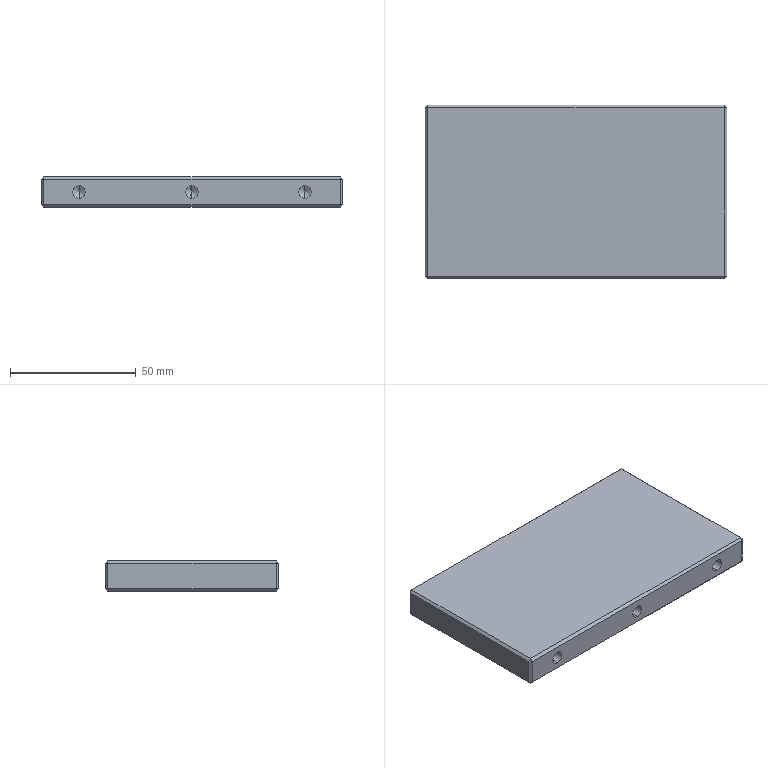Part | STEP file | 06-01-07 support plate | 1 solid | 49 faces | box 120 x 69 x 12 mm | volume 97250 mm3 | plane 27 | cylinder 12 | cone 10 | commonest cylinder face diameters 5 x6 4.2 x4 6 x2
STEP:
#1=CARTESIAN_POINT('',(0.,24.5,3.));
#2=VERTEX_POINT('',#1);
#3=CARTESIAN_POINT('',(0.,24.5,9.));
#4=VERTEX_POINT('',#3);
#5=CARTESIAN_POINT('',(0.,24.5,6.));
#6=DIRECTION('',(0.,1.,0.));
#7=DIRECTION('',(0.,0.,1.));
#8=AXIS2_PLACEMENT_3D('',#5,#6,#7);
#9=CIRCLE('',#8,3.);
#10=EDGE_CURVE('',#2,#4,#9,.T.);
#11=ORIENTED_EDGE('',*,*,#10,.F.);
#12=CARTESIAN_POINT('',(0.,34.5,3.));
#13=VERTEX_POINT('',#12);
#14=CARTESIAN_POINT('',(0.,24.5,3.));
#15=DIRECTION('',(0.,1.,0.));
#16=VECTOR('',#15,1000.);
#17=LINE('',#14,#16);
#18=EDGE_CURVE('',#2,#13,#17,.T.);
#19=ORIENTED_EDGE('',*,*,#18,.T.);
#20=CARTESIAN_POINT('',(0.,34.5,9.));
#21=VERTEX_POINT('',#20);
#22=CARTESIAN_POINT('',(0.,34.5,6.));
#23=DIRECTION('',(0.,1.,0.));
#24=DIRECTION('',(0.,0.,1.));
#25=AXIS2_PLACEMENT_3D('',#22,#23,#24);
#26=CIRCLE('',#25,3.);
#27=EDGE_CURVE('',#13,#21,#26,.T.);
#28=ORIENTED_EDGE('',*,*,#27,.T.);
#29=CARTESIAN_POINT('',(0.,24.5,9.));
#30=DIRECTION('',(0.,1.,0.));
#31=VECTOR('',#30,1000.);
#32=LINE('',#29,#31);
#33=EDGE_CURVE('',#4,#21,#32,.T.);
#34=ORIENTED_EDGE('',*,*,#33,.F.);
#35=EDGE_LOOP('',(#11,#19,#28,#34));
#36=FACE_OUTER_BOUND('',#35,.T.);
#37=CARTESIAN_POINT('',(0.,24.5,6.));
#38=DIRECTION('',(0.,1.,0.));
#39=DIRECTION('',(0.,0.,1.));
#40=AXIS2_PLACEMENT_3D('',#37,#38,#39);
#41=CYLINDRICAL_SURFACE('',#40,3.);
#42=ADVANCED_FACE('',(#36),#41,.F.);
#43=CARTESIAN_POINT('',(-14.5,20.5,3.9));
#44=VERTEX_POINT('',#43);
#45=CARTESIAN_POINT('',(-14.5,20.5,8.1));
#46=VERTEX_POINT('',#45);
#47=CARTESIAN_POINT('',(-14.5,20.5,6.));
#48=DIRECTION('',(0.,1.,0.));
#49=DIRECTION('',(0.,0.,1.));
#50=AXIS2_PLACEMENT_3D('',#47,#48,#49);
#51=CIRCLE('',#50,2.1);
#52=EDGE_CURVE('',#44,#46,#51,.T.);
#53=ORIENTED_EDGE('',*,*,#52,.F.);
#54=CARTESIAN_POINT('',(-14.5,34.5,3.9));
#55=VERTEX_POINT('',#54);
#56=CARTESIAN_POINT('',(-14.5,34.5,3.9));
#57=DIRECTION('',(0.,1.,0.));
#58=VECTOR('',#57,1000.);
#59=LINE('',#56,#58);
#60=EDGE_CURVE('',#44,#55,#59,.T.);
#61=ORIENTED_EDGE('',*,*,#60,.T.);
#62=CARTESIAN_POINT('',(-14.5,34.5,8.1));
#63=VERTEX_POINT('',#62);
#64=CARTESIAN_POINT('',(-14.5,34.5,6.));
#65=DIRECTION('',(0.,1.,0.));
#66=DIRECTION('',(0.,0.,1.));
#67=AXIS2_PLACEMENT_3D('',#64,#65,#66);
#68=CIRCLE('',#67,2.1);
#69=EDGE_CURVE('',#55,#63,#68,.T.);
#70=ORIENTED_EDGE('',*,*,#69,.T.);
#71=CARTESIAN_POINT('',(-14.5,34.5,8.1));
#72=DIRECTION('',(0.,1.,0.));
#73=VECTOR('',#72,1000.);
#74=LINE('',#71,#73);
#75=EDGE_CURVE('',#46,#63,#74,.T.);
#76=ORIENTED_EDGE('',*,*,#75,.F.);
#77=EDGE_LOOP('',(#53,#61,#70,#76));
#78=FACE_OUTER_BOUND('',#77,.T.);
#79=CARTESIAN_POINT('',(-14.5,34.5,6.));
#80=DIRECTION('',(0.,1.,0.));
#81=DIRECTION('',(0.,0.,1.));
#82=AXIS2_PLACEMENT_3D('',#79,#80,#81);
#83=CYLINDRICAL_SURFACE('',#82,2.1);
#84=ADVANCED_FACE('',(#78),#83,.F.);
#85=CARTESIAN_POINT('',(-14.5,19.238,6.));
#86=VERTEX_POINT('',#85);
#87=CARTESIAN_POINT('',(-14.5,20.5,8.1));
#88=DIRECTION('',(0.,0.515,0.8572));
#89=VECTOR('',#88,1000.);
#90=LINE('',#87,#89);
#91=EDGE_CURVE('',#86,#46,#90,.T.);
#92=ORIENTED_EDGE('',*,*,#91,.F.);
#93=CARTESIAN_POINT('',(-14.5,20.5,3.9));
#94=DIRECTION('',(0.,0.515,-0.8572));
#95=VECTOR('',#94,1000.);
#96=LINE('',#93,#95);
#97=EDGE_CURVE('',#86,#44,#96,.T.);
#98=ORIENTED_EDGE('',*,*,#97,.T.);
#99=ORIENTED_EDGE('',*,*,#52,.T.);
#100=EDGE_LOOP('',(#92,#98,#99));
#101=FACE_OUTER_BOUND('',#100,.T.);
#102=CARTESIAN_POINT('',(-14.5,20.5,6.));
#103=DIRECTION('',(0.,1.,0.));
#104=DIRECTION('',(0.,0.,1.));
#105=AXIS2_PLACEMENT_3D('',#102,#103,#104);
#106=CONICAL_SURFACE('',#105,2.1,1.03);
#107=ADVANCED_FACE('',(#101),#106,.F.);
#108=CARTESIAN_POINT('',(45.,20.5,3.9));
#109=VERTEX_POINT('',#108);
#110=CARTESIAN_POINT('',(45.,20.5,8.1));
#111=VERTEX_POINT('',#110);
#112=CARTESIAN_POINT('',(45.,20.5,6.));
#113=DIRECTION('',(0.,1.,0.));
#114=DIRECTION('',(0.,0.,1.));
#115=AXIS2_PLACEMENT_3D('',#112,#113,#114);
#116=CIRCLE('',#115,2.1);
#117=EDGE_CURVE('',#109,#111,#116,.T.);
#118=ORIENTED_EDGE('',*,*,#117,.F.);
#119=CARTESIAN_POINT('',(45.,34.5,3.9));
#120=VERTEX_POINT('',#119);
#121=CARTESIAN_POINT('',(45.,34.5,3.9));
#122=DIRECTION('',(0.,1.,0.));
#123=VECTOR('',#122,1000.);
#124=LINE('',#121,#123);
#125=EDGE_CURVE('',#109,#120,#124,.T.);
#126=ORIENTED_EDGE('',*,*,#125,.T.);
#127=CARTESIAN_POINT('',(45.,34.5,8.1));
#128=VERTEX_POINT('',#127);
#129=CARTESIAN_POINT('',(45.,34.5,6.));
#130=DIRECTION('',(0.,1.,0.));
#131=DIRECTION('',(0.,0.,1.));
#132=AXIS2_PLACEMENT_3D('',#129,#130,#131);
#133=CIRCLE('',#132,2.1);
#134=EDGE_CURVE('',#120,#128,#133,.T.);
#135=ORIENTED_EDGE('',*,*,#134,.T.);
#136=CARTESIAN_POINT('',(45.,34.5,8.1));
#137=DIRECTION('',(0.,1.,0.));
#138=VECTOR('',#137,1000.);
#139=LINE('',#136,#138);
#140=EDGE_CURVE('',#111,#128,#139,.T.);
#141=ORIENTED_EDGE('',*,*,#140,.F.);
#142=EDGE_LOOP('',(#118,#126,#135,#141));
#143=FACE_OUTER_BOUND('',#142,.T.);
#144=CARTESIAN_POINT('',(45.,34.5,6.));
#145=DIRECTION('',(0.,1.,0.));
#146=DIRECTION('',(0.,0.,1.));
#147=AXIS2_PLACEMENT_3D('',#144,#145,#146);
#148=CYLINDRICAL_SURFACE('',#147,2.1);
#149=ADVANCED_FACE('',(#143),#148,.F.);
#150=CARTESIAN_POINT('',(45.,19.238,6.));
#151=VERTEX_POINT('',#150);
#152=CARTESIAN_POINT('',(45.,20.5,8.1));
#153=DIRECTION('',(0.,0.515,0.8572));
#154=VECTOR('',#153,1000.);
#155=LINE('',#152,#154);
#156=EDGE_CURVE('',#151,#111,#155,.T.);
#157=ORIENTED_EDGE('',*,*,#156,.F.);
#158=CARTESIAN_POINT('',(45.,20.5,3.9));
#159=DIRECTION('',(0.,0.515,-0.8572));
#160=VECTOR('',#159,1000.);
#161=LINE('',#158,#160);
#162=EDGE_CURVE('',#151,#109,#161,.T.);
#163=ORIENTED_EDGE('',*,*,#162,.T.);
#164=ORIENTED_EDGE('',*,*,#117,.T.);
#165=EDGE_LOOP('',(#157,#163,#164));
#166=FACE_OUTER_BOUND('',#165,.T.);
#167=CARTESIAN_POINT('',(45.,20.5,6.));
#168=DIRECTION('',(0.,1.,0.));
#169=DIRECTION('',(0.,0.,1.));
#170=AXIS2_PLACEMENT_3D('',#167,#168,#169);
#171=CONICAL_SURFACE('',#170,2.1,1.03);
#172=ADVANCED_FACE('',(#166),#171,.F.);
#173=CARTESIAN_POINT('',(-45.,-17.5,8.5));
#174=VERTEX_POINT('',#173);
#175=CARTESIAN_POINT('',(-45.,-17.5,3.5));
#176=VERTEX_POINT('',#175);
#177=CARTESIAN_POINT('',(-45.,-17.5,6.));
#178=DIRECTION('',(0.,-1.,0.));
#179=DIRECTION('',(0.,0.,-1.));
#180=AXIS2_PLACEMENT_3D('',#177,#178,#179);
#181=CIRCLE('',#180,2.5);
#182=EDGE_CURVE('',#174,#176,#181,.T.);
#183=ORIENTED_EDGE('',*,*,#182,.F.);
#184=CARTESIAN_POINT('',(-45.,-34.5,8.5));
#185=VERTEX_POINT('',#184);
#186=CARTESIAN_POINT('',(-45.,-34.5,8.5));
#187=DIRECTION('',(0.,-1.,0.));
#188=VECTOR('',#187,1000.);
#189=LINE('',#186,#188);
#190=EDGE_CURVE('',#174,#185,#189,.T.);
#191=ORIENTED_EDGE('',*,*,#190,.T.);
#192=CARTESIAN_POINT('',(-45.,-34.5,3.5));
#193=VERTEX_POINT('',#192);
#194=CARTESIAN_POINT('',(-45.,-34.5,6.));
#195=DIRECTION('',(0.,-1.,0.));
#196=DIRECTION('',(0.,0.,-1.));
#197=AXIS2_PLACEMENT_3D('',#194,#195,#196);
#198=CIRCLE('',#197,2.5);
#199=EDGE_CURVE('',#185,#193,#198,.T.);
#200=ORIENTED_EDGE('',*,*,#199,.T.);
#201=CARTESIAN_POINT('',(-45.,-34.5,3.5));
#202=DIRECTION('',(0.,-1.,0.));
#203=VECTOR('',#202,1000.);
#204=LINE('',#201,#203);
#205=EDGE_CURVE('',#176,#193,#204,.T.);
#206=ORIENTED_EDGE('',*,*,#205,.F.);
#207=EDGE_LOOP('',(#183,#191,#200,#206));
#208=FACE_OUTER_BOUND('',#207,.T.);
#209=CARTESIAN_POINT('',(-45.,-34.5,6.));
#210=DIRECTION('',(0.,-1.,0.));
#211=DIRECTION('',(0.,0.,-1.));
#212=AXIS2_PLACEMENT_3D('',#209,#210,#211);
#213=CYLINDRICAL_SURFACE('',#212,2.5);
#214=ADVANCED_FACE('',(#208),#213,.F.);
#215=CARTESIAN_POINT('',(-45.,-15.998,6.));
#216=VERTEX_POINT('',#215);
#217=CARTESIAN_POINT('',(-45.,-17.5,3.5));
#218=DIRECTION('',(0.,-0.515,-0.8572));
#219=VECTOR('',#218,1000.);
#220=LINE('',#217,#219);
#221=EDGE_CURVE('',#216,#176,#220,.T.);
#222=ORIENTED_EDGE('',*,*,#221,.F.);
#223=CARTESIAN_POINT('',(-45.,-17.5,8.5));
#224=DIRECTION('',(0.,-0.515,0.8572));
#225=VECTOR('',#224,1000.);
#226=LINE('',#223,#225);
#227=EDGE_CURVE('',#216,#174,#226,.T.);
#228=ORIENTED_EDGE('',*,*,#227,.T.);
#229=ORIENTED_EDGE('',*,*,#182,.T.);
#230=EDGE_LOOP('',(#222,#228,#229));
#231=FACE_OUTER_BOUND('',#230,.T.);
#232=CARTESIAN_POINT('',(-45.,-17.5,6.));
#233=DIRECTION('',(0.,-1.,0.));
#234=DIRECTION('',(0.,0.,-1.));
#235=AXIS2_PLACEMENT_3D('',#232,#233,#234);
#236=CONICAL_SURFACE('',#235,2.5,1.03);
#237=ADVANCED_FACE('',(#231),#236,.F.);
#238=CARTESIAN_POINT('',(0.,-17.5,8.5));
#239=VERTEX_POINT('',#238);
#240=CARTESIAN_POINT('',(0.,-17.5,3.5));
#241=VERTEX_POINT('',#240);
#242=CARTESIAN_POINT('',(0.,-17.5,6.));
#243=DIRECTION('',(0.,-1.,0.));
#244=DIRECTION('',(0.,0.,-1.));
#245=AXIS2_PLACEMENT_3D('',#242,#243,#244);
#246=CIRCLE('',#245,2.5);
#247=EDGE_CURVE('',#239,#241,#246,.T.);
#248=ORIENTED_EDGE('',*,*,#247,.F.);
#249=CARTESIAN_POINT('',(0.,-34.5,8.5));
#250=VERTEX_POINT('',#249);
#251=CARTESIAN_POINT('',(0.,-34.5,8.5));
#252=DIRECTION('',(0.,-1.,0.));
#253=VECTOR('',#252,1000.);
#254=LINE('',#251,#253);
#255=EDGE_CURVE('',#239,#250,#254,.T.);
#256=ORIENTED_EDGE('',*,*,#255,.T.);
#257=CARTESIAN_POINT('',(0.,-34.5,3.5));
#258=VERTEX_POINT('',#257);
#259=CARTESIAN_POINT('',(0.,-34.5,6.));
#260=DIRECTION('',(0.,-1.,0.));
#261=DIRECTION('',(0.,0.,-1.));
#262=AXIS2_PLACEMENT_3D('',#259,#260,#261);
#263=CIRCLE('',#262,2.5);
#264=EDGE_CURVE('',#250,#258,#263,.T.);
#265=ORIENTED_EDGE('',*,*,#264,.T.);
#266=CARTESIAN_POINT('',(0.,-34.5,3.5));
#267=DIRECTION('',(0.,-1.,0.));
#268=VECTOR('',#267,1000.);
#269=LINE('',#266,#268);
#270=EDGE_CURVE('',#241,#258,#269,.T.);
#271=ORIENTED_EDGE('',*,*,#270,.F.);
#272=EDGE_LOOP('',(#248,#256,#265,#271));
#273=FACE_OUTER_BOUND('',#272,.T.);
#274=CARTESIAN_POINT('',(0.,-34.5,6.));
#275=DIRECTION('',(0.,-1.,0.));
#276=DIRECTION('',(0.,0.,-1.));
#277=AXIS2_PLACEMENT_3D('',#274,#275,#276);
#278=CYLINDRICAL_SURFACE('',#277,2.5);
#279=ADVANCED_FACE('',(#273),#278,.F.);
#280=CARTESIAN_POINT('',(0.,-15.998,6.));
#281=VERTEX_POINT('',#280);
#282=CARTESIAN_POINT('',(0.,-17.5,3.5));
#283=DIRECTION('',(0.,-0.515,-0.8572));
#284=VECTOR('',#283,1000.);
#285=LINE('',#282,#284);
#286=EDGE_CURVE('',#281,#241,#285,.T.);
#287=ORIENTED_EDGE('',*,*,#286,.F.);
#288=CARTESIAN_POINT('',(0.,-17.5,8.5));
#289=DIRECTION('',(0.,-0.515,0.8572));
#290=VECTOR('',#289,1000.);
#291=LINE('',#288,#290);
#292=EDGE_CURVE('',#281,#239,#291,.T.);
#293=ORIENTED_EDGE('',*,*,#292,.T.);
#294=ORIENTED_EDGE('',*,*,#247,.T.);
#295=EDGE_LOOP('',(#287,#293,#294));
#296=FACE_OUTER_BOUND('',#295,.T.);
#297=CARTESIAN_POINT('',(0.,-17.5,6.));
#298=DIRECTION('',(0.,-1.,0.));
#299=DIRECTION('',(0.,0.,-1.));
#300=AXIS2_PLACEMENT_3D('',#297,#298,#299);
#301=CONICAL_SURFACE('',#300,2.5,1.03);
#302=ADVANCED_FACE('',(#296),#301,.F.);
#303=CARTESIAN_POINT('',(45.,-17.5,8.5));
#304=VERTEX_POINT('',#303);
#305=CARTESIAN_POINT('',(45.,-17.5,3.5));
#306=VERTEX_POINT('',#305);
#307=CARTESIAN_POINT('',(45.,-17.5,6.));
#308=DIRECTION('',(0.,-1.,0.));
#309=DIRECTION('',(0.,0.,-1.));
#310=AXIS2_PLACEMENT_3D('',#307,#308,#309);
#311=CIRCLE('',#310,2.5);
#312=EDGE_CURVE('',#304,#306,#311,.T.);
#313=ORIENTED_EDGE('',*,*,#312,.F.);
#314=CARTESIAN_POINT('',(45.,-34.5,8.5));
#315=VERTEX_POINT('',#314);
#316=CARTESIAN_POINT('',(45.,-34.5,8.5));
#317=DIRECTION('',(0.,-1.,0.));
#318=VECTOR('',#317,1000.);
#319=LINE('',#316,#318);
#320=EDGE_CURVE('',#304,#315,#319,.T.);
#321=ORIENTED_EDGE('',*,*,#320,.T.);
#322=CARTESIAN_POINT('',(45.,-34.5,3.5));
#323=VERTEX_POINT('',#322);
#324=CARTESIAN_POINT('',(45.,-34.5,6.));
#325=DIRECTION('',(0.,-1.,0.));
#326=DIRECTION('',(0.,0.,-1.));
#327=AXIS2_PLACEMENT_3D('',#324,#325,#326);
#328=CIRCLE('',#327,2.5);
#329=EDGE_CURVE('',#315,#323,#328,.T.);
#330=ORIENTED_EDGE('',*,*,#329,.T.);
#331=CARTESIAN_POINT('',(45.,-34.5,3.5));
#332=DIRECTION('',(0.,-1.,0.));
#333=VECTOR('',#332,1000.);
#334=LINE('',#331,#333);
#335=EDGE_CURVE('',#306,#323,#334,.T.);
#336=ORIENTED_EDGE('',*,*,#335,.F.);
#337=EDGE_LOOP('',(#313,#321,#330,#336));
#338=FACE_OUTER_BOUND('',#337,.T.);
#339=CARTESIAN_POINT('',(45.,-34.5,6.));
#340=DIRECTION('',(0.,-1.,0.));
#341=DIRECTION('',(0.,0.,-1.));
#342=AXIS2_PLACEMENT_3D('',#339,#340,#341);
#343=CYLINDRICAL_SURFACE('',#342,2.5);
#344=ADVANCED_FACE('',(#338),#343,.F.);
#345=CARTESIAN_POINT('',(45.,-15.998,6.));
#346=VERTEX_POINT('',#345);
#347=CARTESIAN_POINT('',(45.,-17.5,3.5));
#348=DIRECTION('',(0.,-0.515,-0.8572));
#349=VECTOR('',#348,1000.);
#350=LINE('',#347,#349);
#351=EDGE_CURVE('',#346,#306,#350,.T.);
#352=ORIENTED_EDGE('',*,*,#351,.F.);
#353=CARTESIAN_POINT('',(45.,-17.5,8.5));
#354=DIRECTION('',(0.,-0.515,0.8572));
#355=VECTOR('',#354,1000.);
#356=LINE('',#353,#355);
#357=EDGE_CURVE('',#346,#304,#356,.T.);
#358=ORIENTED_EDGE('',*,*,#357,.T.);
#359=ORIENTED_EDGE('',*,*,#312,.T.);
#360=EDGE_LOOP('',(#352,#358,#359));
#361=FACE_OUTER_BOUND('',#360,.T.);
#362=CARTESIAN_POINT('',(45.,-17.5,6.));
#363=DIRECTION('',(0.,-1.,0.));
#364=DIRECTION('',(0.,0.,-1.));
#365=AXIS2_PLACEMENT_3D('',#362,#363,#364);
#366=CONICAL_SURFACE('',#365,2.5,1.03);
#367=ADVANCED_FACE('',(#361),#366,.F.);
#368=CARTESIAN_POINT('',(60.,-33.5,11.));
#369=VERTEX_POINT('',#368);
#370=CARTESIAN_POINT('',(60.,-33.5,1.));
#371=VERTEX_POINT('',#370);
#372=CARTESIAN_POINT('',(60.,-33.5,12.));
#373=DIRECTION('',(0.,0.,-1.));
#374=VECTOR('',#373,1000.);
#375=LINE('',#372,#374);
#376=EDGE_CURVE('',#369,#371,#375,.T.);
#377=ORIENTED_EDGE('',*,*,#376,.T.);
#378=CARTESIAN_POINT('',(60.,33.5,1.));
#379=VERTEX_POINT('',#378);
#380=CARTESIAN_POINT('',(60.,34.5,1.));
#381=DIRECTION('',(0.,1.,0.));
#382=VECTOR('',#381,1000.);
#383=LINE('',#380,#382);
#384=EDGE_CURVE('',#371,#379,#383,.T.);
#385=ORIENTED_EDGE('',*,*,#384,.T.);
#386=CARTESIAN_POINT('',(60.,33.5,11.));
#387=VERTEX_POINT('',#386);
#388=CARTESIAN_POINT('',(60.,33.5,12.));
#389=DIRECTION('',(0.,0.,1.));
#390=VECTOR('',#389,1000.);
#391=LINE('',#388,#390);
#392=EDGE_CURVE('',#379,#387,#391,.T.);
#393=ORIENTED_EDGE('',*,*,#392,.T.);
#394=CARTESIAN_POINT('',(60.,-34.5,11.));
#395=DIRECTION('',(0.,-1.,0.));
#396=VECTOR('',#395,1000.);
#397=LINE('',#394,#396);
#398=EDGE_CURVE('',#387,#369,#397,.T.);
#399=ORIENTED_EDGE('',*,*,#398,.T.);
#400=EDGE_LOOP('',(#377,#385,#393,#399));
#401=FACE_OUTER_BOUND('',#400,.T.);
#402=CARTESIAN_POINT('',(60.,34.5,12.));
#403=DIRECTION('',(-1.,0.,0.));
#404=DIRECTION('',(0.,-1.,0.));
#405=AXIS2_PLACEMENT_3D('',#402,#403,#404);
#406=PLANE('',#405);
#407=ADVANCED_FACE('',(#401),#406,.F.);
#408=CARTESIAN_POINT('',(59.,34.5,11.));
#409=VERTEX_POINT('',#408);
#410=CARTESIAN_POINT('',(59.,34.5,1.));
#411=VERTEX_POINT('',#410);
#412=CARTESIAN_POINT('',(59.,34.5,12.));
#413=DIRECTION('',(0.,0.,-1.));
#414=VECTOR('',#413,1000.);
#415=LINE('',#412,#414);
#416=EDGE_CURVE('',#409,#411,#415,.T.);
#417=ORIENTED_EDGE('',*,*,#416,.T.);
#418=CARTESIAN_POINT('',(-59.,34.5,1.));
#419=VERTEX_POINT('',#418);
#420=CARTESIAN_POINT('',(-60.,34.5,1.));
#421=DIRECTION('',(-1.,0.,0.));
#422=VECTOR('',#421,1000.);
#423=LINE('',#420,#422);
#424=EDGE_CURVE('',#411,#419,#423,.T.);
#425=ORIENTED_EDGE('',*,*,#424,.T.);
#426=CARTESIAN_POINT('',(-59.,34.5,11.));
#427=VERTEX_POINT('',#426);
#428=CARTESIAN_POINT('',(-59.,34.5,12.));
#429=DIRECTION('',(0.,0.,1.));
#430=VECTOR('',#429,1000.);
#431=LINE('',#428,#430);
#432=EDGE_CURVE('',#419,#427,#431,.T.);
#433=ORIENTED_EDGE('',*,*,#432,.T.);
#434=CARTESIAN_POINT('',(60.,34.5,11.));
#435=DIRECTION('',(1.,0.,0.));
#436=VECTOR('',#435,1000.);
#437=LINE('',#434,#436);
#438=EDGE_CURVE('',#427,#409,#437,.T.);
#439=ORIENTED_EDGE('',*,*,#438,.T.);
#440=EDGE_LOOP('',(#417,#425,#433,#439));
#441=FACE_OUTER_BOUND('',#440,.T.);
#442=CARTESIAN_POINT('',(0.,34.5,6.));
#443=DIRECTION('',(0.,1.,0.));
#444=DIRECTION('',(0.,0.,1.));
#445=AXIS2_PLACEMENT_3D('',#442,#443,#444);
#446=CIRCLE('',#445,3.);
#447=EDGE_CURVE('',#21,#13,#446,.T.);
#448=ORIENTED_EDGE('',*,*,#447,.F.);
#449=ORIENTED_EDGE('',*,*,#27,.F.);
#450=EDGE_LOOP('',(#448,#449));
#451=FACE_BOUND('',#450,.T.);
#452=CARTESIAN_POINT('',(-14.5,34.5,6.));
#453=DIRECTION('',(0.,1.,0.));
#454=DIRECTION('',(0.,0.,1.));
#455=AXIS2_PLACEMENT_3D('',#452,#453,#454);
#456=CIRCLE('',#455,2.1);
#457=EDGE_CURVE('',#63,#55,#456,.T.);
#458=ORIENTED_EDGE('',*,*,#457,.F.);
#459=ORIENTED_EDGE('',*,*,#69,.F.);
#460=EDGE_LOOP('',(#458,#459));
#461=FACE_BOUND('',#460,.T.);
#462=CARTESIAN_POINT('',(45.,34.5,6.));
#463=DIRECTION('',(0.,1.,0.));
#464=DIRECTION('',(0.,0.,1.));
#465=AXIS2_PLACEMENT_3D('',#462,#463,#464);
#466=CIRCLE('',#465,2.1);
#467=EDGE_CURVE('',#128,#120,#466,.T.);
#468=ORIENTED_EDGE('',*,*,#467,.F.);
#469=ORIENTED_EDGE('',*,*,#134,.F.);
#470=EDGE_LOOP('',(#468,#469));
#471=FACE_BOUND('',#470,.T.);
#472=CARTESIAN_POINT('',(-60.,34.5,12.));
#473=DIRECTION('',(0.,-1.,0.));
#474=DIRECTION('',(0.,0.,-1.));
#475=AXIS2_PLACEMENT_3D('',#472,#473,#474);
#476=PLANE('',#475);
#477=ADVANCED_FACE('',(#441,#451,#461,#471),#476,.F.);
#478=CARTESIAN_POINT('',(-60.,33.5,11.));
#479=VERTEX_POINT('',#478);
#480=CARTESIAN_POINT('',(-60.,33.5,1.));
#481=VERTEX_POINT('',#480);
#482=CARTESIAN_POINT('',(-60.,33.5,12.));
#483=DIRECTION('',(0.,0.,-1.));
#484=VECTOR('',#483,1000.);
#485=LINE('',#482,#484);
#486=EDGE_CURVE('',#479,#481,#485,.T.);
#487=ORIENTED_EDGE('',*,*,#486,.T.);
#488=CARTESIAN_POINT('',(-60.,-33.5,1.));
#489=VERTEX_POINT('',#488);
#490=CARTESIAN_POINT('',(-60.,34.5,1.));
#491=DIRECTION('',(0.,-1.,0.));
#492=VECTOR('',#491,1000.);
#493=LINE('',#490,#492);
#494=EDGE_CURVE('',#481,#489,#493,.T.);
#495=ORIENTED_EDGE('',*,*,#494,.T.);
#496=CARTESIAN_POINT('',(-60.,-33.5,11.));
#497=VERTEX_POINT('',#496);
#498=CARTESIAN_POINT('',(-60.,-33.5,12.));
#499=DIRECTION('',(0.,0.,1.));
#500=VECTOR('',#499,1000.);
#501=LINE('',#498,#500);
#502=EDGE_CURVE('',#489,#497,#501,.T.);
#503=ORIENTED_EDGE('',*,*,#502,.T.);
#504=CARTESIAN_POINT('',(-60.,34.5,11.));
#505=DIRECTION('',(0.,1.,0.));
#506=VECTOR('',#505,1000.);
#507=LINE('',#504,#506);
#508=EDGE_CURVE('',#497,#479,#507,.T.);
#509=ORIENTED_EDGE('',*,*,#508,.T.);
#510=EDGE_LOOP('',(#487,#495,#503,#509));
#511=FACE_OUTER_BOUND('',#510,.T.);
#512=CARTESIAN_POINT('',(-60.,34.5,12.));
#513=DIRECTION('',(1.,0.,0.));
#514=DIRECTION('',(0.,1.,0.));
#515=AXIS2_PLACEMENT_3D('',#512,#513,#514);
#516=PLANE('',#515);
#517=ADVANCED_FACE('',(#511),#516,.F.);
#518=CARTESIAN_POINT('',(59.,-34.5,11.));
#519=VERTEX_POINT('',#518);
#520=CARTESIAN_POINT('',(-59.,-34.5,11.));
#521=VERTEX_POINT('',#520);
#522=CARTESIAN_POINT('',(-60.,-34.5,11.));
#523=DIRECTION('',(-1.,0.,0.));
#524=VECTOR('',#523,1000.);
#525=LINE('',#522,#524);
#526=EDGE_CURVE('',#519,#521,#525,.T.);
#527=ORIENTED_EDGE('',*,*,#526,.T.);
#528=CARTESIAN_POINT('',(-59.,-34.5,1.));
#529=VERTEX_POINT('',#528);
#530=CARTESIAN_POINT('',(-59.,-34.5,12.));
#531=DIRECTION('',(0.,0.,-1.));
#532=VECTOR('',#531,1000.);
#533=LINE('',#530,#532);
#534=EDGE_CURVE('',#521,#529,#533,.T.);
#535=ORIENTED_EDGE('',*,*,#534,.T.);
#536=CARTESIAN_POINT('',(59.,-34.5,1.));
#537=VERTEX_POINT('',#536);
#538=CARTESIAN_POINT('',(-60.,-34.5,1.));
#539=DIRECTION('',(1.,0.,0.));
#540=VECTOR('',#539,1000.);
#541=LINE('',#538,#540);
#542=EDGE_CURVE('',#529,#537,#541,.T.);
#543=ORIENTED_EDGE('',*,*,#542,.T.);
#544=CARTESIAN_POINT('',(59.,-34.5,12.));
#545=DIRECTION('',(0.,0.,1.));
#546=VECTOR('',#545,1000.);
#547=LINE('',#544,#546);
#548=EDGE_CURVE('',#537,#519,#547,.T.);
#549=ORIENTED_EDGE('',*,*,#548,.T.);
#550=EDGE_LOOP('',(#527,#535,#543,#549));
#551=FACE_OUTER_BOUND('',#550,.T.);
#552=CARTESIAN_POINT('',(-45.,-34.5,6.));
#553=DIRECTION('',(0.,-1.,0.));
#554=DIRECTION('',(0.,0.,-1.));
#555=AXIS2_PLACEMENT_3D('',#552,#553,#554);
#556=CIRCLE('',#555,2.5);
#557=EDGE_CURVE('',#193,#185,#556,.T.);
#558=ORIENTED_EDGE('',*,*,#557,.F.);
#559=ORIENTED_EDGE('',*,*,#199,.F.);
#560=EDGE_LOOP('',(#558,#559));
#561=FACE_BOUND('',#560,.T.);
#562=CARTESIAN_POINT('',(0.,-34.5,6.));
#563=DIRECTION('',(0.,-1.,0.));
#564=DIRECTION('',(0.,0.,-1.));
#565=AXIS2_PLACEMENT_3D('',#562,#563,#564);
#566=CIRCLE('',#565,2.5);
#567=EDGE_CURVE('',#258,#250,#566,.T.);
#568=ORIENTED_EDGE('',*,*,#567,.F.);
#569=ORIENTED_EDGE('',*,*,#264,.F.);
#570=EDGE_LOOP('',(#568,#569));
#571=FACE_BOUND('',#570,.T.);
#572=CARTESIAN_POINT('',(45.,-34.5,6.));
#573=DIRECTION('',(0.,-1.,0.));
#574=DIRECTION('',(0.,0.,-1.));
#575=AXIS2_PLACEMENT_3D('',#572,#573,#574);
#576=CIRCLE('',#575,2.5);
#577=EDGE_CURVE('',#323,#315,#576,.T.);
#578=ORIENTED_EDGE('',*,*,#577,.F.);
#579=ORIENTED_EDGE('',*,*,#329,.F.);
#580=EDGE_LOOP('',(#578,#579));
#581=FACE_BOUND('',#580,.T.);
#582=CARTESIAN_POINT('',(-60.,-34.5,12.));
#583=DIRECTION('',(0.,1.,0.));
#584=DIRECTION('',(0.,0.,1.));
#585=AXIS2_PLACEMENT_3D('',#582,#583,#584);
#586=PLANE('',#585);
#587=ADVANCED_FACE('',(#551,#561,#571,#581),#586,.F.);
#588=CARTESIAN_POINT('',(-59.,33.5,12.));
#589=VERTEX_POINT('',#588);
#590=CARTESIAN_POINT('',(-59.,-33.5,12.));
#591=VERTEX_POINT('',#590);
#592=CARTESIAN_POINT('',(-59.,-34.5,12.));
#593=DIRECTION('',(0.,-1.,0.));
#594=VECTOR('',#593,1000.);
#595=LINE('',#592,#594);
#596=EDGE_CURVE('',#589,#591,#595,.T.);
#597=ORIENTED_EDGE('',*,*,#596,.T.);
#598=CARTESIAN_POINT('',(59.,-33.5,12.));
#599=VERTEX_POINT('',#598);
#600=CARTESIAN_POINT('',(60.,-33.5,12.));
#601=DIRECTION('',(1.,0.,0.));
#602=VECTOR('',#601,1000.);
#603=LINE('',#600,#602);
#604=EDGE_CURVE('',#591,#599,#603,.T.);
#605=ORIENTED_EDGE('',*,*,#604,.T.);
#606=CARTESIAN_POINT('',(59.,33.5,12.));
#607=VERTEX_POINT('',#606);
#608=CARTESIAN_POINT('',(59.,34.5,12.));
#609=DIRECTION('',(0.,1.,0.));
#610=VECTOR('',#609,1000.);
#611=LINE('',#608,#610);
#612=EDGE_CURVE('',#599,#607,#611,.T.);
#613=ORIENTED_EDGE('',*,*,#612,.T.);
#614=CARTESIAN_POINT('',(-60.,33.5,12.));
#615=DIRECTION('',(-1.,0.,0.));
#616=VECTOR('',#615,1000.);
#617=LINE('',#614,#616);
#618=EDGE_CURVE('',#607,#589,#617,.T.);
#619=ORIENTED_EDGE('',*,*,#618,.T.);
#620=EDGE_LOOP('',(#597,#605,#613,#619));
#621=FACE_OUTER_BOUND('',#620,.T.);
#622=CARTESIAN_POINT('',(60.,-34.5,12.));
#623=DIRECTION('',(0.,0.,1.));
#624=DIRECTION('',(1.,0.,0.));
#625=AXIS2_PLACEMENT_3D('',#622,#623,#624);
#626=PLANE('',#625);
#627=ADVANCED_FACE('',(#621),#626,.T.);
#628=CARTESIAN_POINT('',(-59.,-33.5,0.));
#629=VERTEX_POINT('',#628);
#630=CARTESIAN_POINT('',(-59.,33.5,0.));
#631=VERTEX_POINT('',#630);
#632=CARTESIAN_POINT('',(-59.,-34.5,0.));
#633=DIRECTION('',(0.,1.,0.));
#634=VECTOR('',#633,1000.);
#635=LINE('',#632,#634);
#636=EDGE_CURVE('',#629,#631,#635,.T.);
#637=ORIENTED_EDGE('',*,*,#636,.T.);
#638=CARTESIAN_POINT('',(59.,33.5,0.));
#639=VERTEX_POINT('',#638);
#640=CARTESIAN_POINT('',(60.,33.5,0.));
#641=DIRECTION('',(1.,0.,0.));
#642=VECTOR('',#641,1000.);
#643=LINE('',#640,#642);
#644=EDGE_CURVE('',#631,#639,#643,.T.);
#645=ORIENTED_EDGE('',*,*,#644,.T.);
#646=CARTESIAN_POINT('',(59.,-33.5,0.));
#647=VERTEX_POINT('',#646);
#648=CARTESIAN_POINT('',(59.,-34.5,0.));
#649=DIRECTION('',(0.,-1.,0.));
#650=VECTOR('',#649,1000.);
#651=LINE('',#648,#650);
#652=EDGE_CURVE('',#639,#647,#651,.T.);
#653=ORIENTED_EDGE('',*,*,#652,.T.);
#654=CARTESIAN_POINT('',(60.,-33.5,0.));
#655=DIRECTION('',(-1.,0.,0.));
#656=VECTOR('',#655,1000.);
#657=LINE('',#654,#656);
#658=EDGE_CURVE('',#647,#629,#657,.T.);
#659=ORIENTED_EDGE('',*,*,#658,.T.);
#660=EDGE_LOOP('',(#637,#645,#653,#659));
#661=FACE_OUTER_BOUND('',#660,.T.);
#662=CARTESIAN_POINT('',(60.,-34.5,0.));
#663=DIRECTION('',(0.,0.,1.));
#664=DIRECTION('',(1.,0.,0.));
#665=AXIS2_PLACEMENT_3D('',#662,#663,#664);
#666=PLANE('',#665);
#667=ADVANCED_FACE('',(#661),#666,.F.);
#668=ORIENTED_EDGE('',*,*,#357,.F.);
#669=ORIENTED_EDGE('',*,*,#351,.T.);
#670=CARTESIAN_POINT('',(45.,-17.5,6.));
#671=DIRECTION('',(0.,-1.,0.));
#672=DIRECTION('',(0.,0.,-1.));
#673=AXIS2_PLACEMENT_3D('',#670,#671,#672);
#674=CIRCLE('',#673,2.5);
#675=EDGE_CURVE('',#306,#304,#674,.T.);
#676=ORIENTED_EDGE('',*,*,#675,.T.);
#677=EDGE_LOOP('',(#668,#669,#676));
#678=FACE_OUTER_BOUND('',#677,.T.);
#679=CARTESIAN_POINT('',(45.,-17.5,6.));
#680=DIRECTION('',(0.,-1.,0.));
#681=DIRECTION('',(0.,0.,-1.));
#682=AXIS2_PLACEMENT_3D('',#679,#680,#681);
#683=CONICAL_SURFACE('',#682,2.5,1.03);
#684=ADVANCED_FACE('',(#678),#683,.F.);
#685=ORIENTED_EDGE('',*,*,#320,.F.);
#686=ORIENTED_EDGE('',*,*,#675,.F.);
#687=ORIENTED_EDGE('',*,*,#335,.T.);
#688=ORIENTED_EDGE('',*,*,#577,.T.);
#689=EDGE_LOOP('',(#685,#686,#687,#688));
#690=FACE_OUTER_BOUND('',#689,.T.);
#691=CARTESIAN_POINT('',(45.,-34.5,6.));
#692=DIRECTION('',(0.,-1.,0.));
#693=DIRECTION('',(0.,0.,-1.));
#694=AXIS2_PLACEMENT_3D('',#691,#692,#693);
#695=CYLINDRICAL_SURFACE('',#694,2.5);
#696=ADVANCED_FACE('',(#690),#695,.F.);
#697=ORIENTED_EDGE('',*,*,#292,.F.);
#698=ORIENTED_EDGE('',*,*,#286,.T.);
#699=CARTESIAN_POINT('',(0.,-17.5,6.));
#700=DIRECTION('',(0.,-1.,0.));
#701=DIRECTION('',(0.,0.,-1.));
#702=AXIS2_PLACEMENT_3D('',#699,#700,#701);
#703=CIRCLE('',#702,2.5);
#704=EDGE_CURVE('',#241,#239,#703,.T.);
#705=ORIENTED_EDGE('',*,*,#704,.T.);
#706=EDGE_LOOP('',(#697,#698,#705));
#707=FACE_OUTER_BOUND('',#706,.T.);
#708=CARTESIAN_POINT('',(0.,-17.5,6.));
#709=DIRECTION('',(0.,-1.,0.));
#710=DIRECTION('',(0.,0.,-1.));
#711=AXIS2_PLACEMENT_3D('',#708,#709,#710);
#712=CONICAL_SURFACE('',#711,2.5,1.03);
#713=ADVANCED_FACE('',(#707),#712,.F.);
#714=ORIENTED_EDGE('',*,*,#255,.F.);
#715=ORIENTED_EDGE('',*,*,#704,.F.);
#716=ORIENTED_EDGE('',*,*,#270,.T.);
#717=ORIENTED_EDGE('',*,*,#567,.T.);
#718=EDGE_LOOP('',(#714,#715,#716,#717));
#719=FACE_OUTER_BOUND('',#718,.T.);
#720=CARTESIAN_POINT('',(0.,-34.5,6.));
#721=DIRECTION('',(0.,-1.,0.));
#722=DIRECTION('',(0.,0.,-1.));
#723=AXIS2_PLACEMENT_3D('',#720,#721,#722);
#724=CYLINDRICAL_SURFACE('',#723,2.5);
#725=ADVANCED_FACE('',(#719),#724,.F.);
#726=ORIENTED_EDGE('',*,*,#227,.F.);
#727=ORIENTED_EDGE('',*,*,#221,.T.);
#728=CARTESIAN_POINT('',(-45.,-17.5,6.));
#729=DIRECTION('',(0.,-1.,0.));
#730=DIRECTION('',(0.,0.,-1.));
#731=AXIS2_PLACEMENT_3D('',#728,#729,#730);
#732=CIRCLE('',#731,2.5);
#733=EDGE_CURVE('',#176,#174,#732,.T.);
#734=ORIENTED_EDGE('',*,*,#733,.T.);
#735=EDGE_LOOP('',(#726,#727,#734));
#736=FACE_OUTER_BOUND('',#735,.T.);
#737=CARTESIAN_POINT('',(-45.,-17.5,6.));
#738=DIRECTION('',(0.,-1.,0.));
#739=DIRECTION('',(0.,0.,-1.));
#740=AXIS2_PLACEMENT_3D('',#737,#738,#739);
#741=CONICAL_SURFACE('',#740,2.5,1.03);
#742=ADVANCED_FACE('',(#736),#741,.F.);
#743=ORIENTED_EDGE('',*,*,#190,.F.);
#744=ORIENTED_EDGE('',*,*,#733,.F.);
#745=ORIENTED_EDGE('',*,*,#205,.T.);
#746=ORIENTED_EDGE('',*,*,#557,.T.);
#747=EDGE_LOOP('',(#743,#744,#745,#746));
#748=FACE_OUTER_BOUND('',#747,.T.);
#749=CARTESIAN_POINT('',(-45.,-34.5,6.));
#750=DIRECTION('',(0.,-1.,0.));
#751=DIRECTION('',(0.,0.,-1.));
#752=AXIS2_PLACEMENT_3D('',#749,#750,#751);
#753=CYLINDRICAL_SURFACE('',#752,2.5);
#754=ADVANCED_FACE('',(#748),#753,.F.);
#755=ORIENTED_EDGE('',*,*,#162,.F.);
#756=ORIENTED_EDGE('',*,*,#156,.T.);
#757=CARTESIAN_POINT('',(45.,20.5,6.));
#758=DIRECTION('',(0.,1.,0.));
#759=DIRECTION('',(0.,0.,1.));
#760=AXIS2_PLACEMENT_3D('',#757,#758,#759);
#761=CIRCLE('',#760,2.1);
#762=EDGE_CURVE('',#111,#109,#761,.T.);
#763=ORIENTED_EDGE('',*,*,#762,.T.);
#764=EDGE_LOOP('',(#755,#756,#763));
#765=FACE_OUTER_BOUND('',#764,.T.);
#766=CARTESIAN_POINT('',(45.,20.5,6.));
#767=DIRECTION('',(0.,1.,0.));
#768=DIRECTION('',(0.,0.,1.));
#769=AXIS2_PLACEMENT_3D('',#766,#767,#768);
#770=CONICAL_SURFACE('',#769,2.1,1.03);
#771=ADVANCED_FACE('',(#765),#770,.F.);
#772=ORIENTED_EDGE('',*,*,#125,.F.);
#773=ORIENTED_EDGE('',*,*,#762,.F.);
#774=ORIENTED_EDGE('',*,*,#140,.T.);
#775=ORIENTED_EDGE('',*,*,#467,.T.);
#776=EDGE_LOOP('',(#772,#773,#774,#775));
#777=FACE_OUTER_BOUND('',#776,.T.);
#778=CARTESIAN_POINT('',(45.,34.5,6.));
#779=DIRECTION('',(0.,1.,0.));
#780=DIRECTION('',(0.,0.,1.));
#781=AXIS2_PLACEMENT_3D('',#778,#779,#780);
#782=CYLINDRICAL_SURFACE('',#781,2.1);
#783=ADVANCED_FACE('',(#777),#782,.F.);
#784=ORIENTED_EDGE('',*,*,#97,.F.);
#785=ORIENTED_EDGE('',*,*,#91,.T.);
#786=CARTESIAN_POINT('',(-14.5,20.5,6.));
#787=DIRECTION('',(0.,1.,0.));
#788=DIRECTION('',(0.,0.,1.));
#789=AXIS2_PLACEMENT_3D('',#786,#787,#788);
#790=CIRCLE('',#789,2.1);
#791=EDGE_CURVE('',#46,#44,#790,.T.);
#792=ORIENTED_EDGE('',*,*,#791,.T.);
#793=EDGE_LOOP('',(#784,#785,#792));
#794=FACE_OUTER_BOUND('',#793,.T.);
#795=CARTESIAN_POINT('',(-14.5,20.5,6.));
#796=DIRECTION('',(0.,1.,0.));
#797=DIRECTION('',(0.,0.,1.));
#798=AXIS2_PLACEMENT_3D('',#795,#796,#797);
#799=CONICAL_SURFACE('',#798,2.1,1.03);
#800=ADVANCED_FACE('',(#794),#799,.F.);
#801=ORIENTED_EDGE('',*,*,#60,.F.);
#802=ORIENTED_EDGE('',*,*,#791,.F.);
#803=ORIENTED_EDGE('',*,*,#75,.T.);
#804=ORIENTED_EDGE('',*,*,#457,.T.);
#805=EDGE_LOOP('',(#801,#802,#803,#804));
#806=FACE_OUTER_BOUND('',#805,.T.);
#807=CARTESIAN_POINT('',(-14.5,34.5,6.));
#808=DIRECTION('',(0.,1.,0.));
#809=DIRECTION('',(0.,0.,1.));
#810=AXIS2_PLACEMENT_3D('',#807,#808,#809);
#811=CYLINDRICAL_SURFACE('',#810,2.1);
#812=ADVANCED_FACE('',(#806),#811,.F.);
#813=ORIENTED_EDGE('',*,*,#18,.F.);
#814=CARTESIAN_POINT('',(0.,24.5,6.));
#815=DIRECTION('',(0.,1.,0.));
#816=DIRECTION('',(0.,0.,1.));
#817=AXIS2_PLACEMENT_3D('',#814,#815,#816);
#818=CIRCLE('',#817,3.);
#819=EDGE_CURVE('',#4,#2,#818,.T.);
#820=ORIENTED_EDGE('',*,*,#819,.F.);
#821=ORIENTED_EDGE('',*,*,#33,.T.);
#822=ORIENTED_EDGE('',*,*,#447,.T.);
#823=EDGE_LOOP('',(#813,#820,#821,#822));
#824=FACE_OUTER_BOUND('',#823,.T.);
#825=CARTESIAN_POINT('',(0.,24.5,6.));
#826=DIRECTION('',(0.,1.,0.));
#827=DIRECTION('',(0.,0.,1.));
#828=AXIS2_PLACEMENT_3D('',#825,#826,#827);
#829=CYLINDRICAL_SURFACE('',#828,3.);
#830=ADVANCED_FACE('',(#824),#829,.F.);
#831=ORIENTED_EDGE('',*,*,#819,.T.);
#832=ORIENTED_EDGE('',*,*,#10,.T.);
#833=EDGE_LOOP('',(#831,#832));
#834=FACE_OUTER_BOUND('',#833,.T.);
#835=CARTESIAN_POINT('',(0.,24.5,6.));
#836=DIRECTION('',(0.,1.,0.));
#837=DIRECTION('',(0.,0.,1.));
#838=AXIS2_PLACEMENT_3D('',#835,#836,#837);
#839=PLANE('',#838);
#840=ADVANCED_FACE('',(#834),#839,.T.);
#841=CARTESIAN_POINT('',(59.,-33.5,12.));
#842=DIRECTION('',(0.,-0.7071,-0.7071));
#843=VECTOR('',#842,1000.);
#844=LINE('',#841,#843);
#845=EDGE_CURVE('',#599,#519,#844,.T.);
#846=ORIENTED_EDGE('',*,*,#845,.F.);
#847=ORIENTED_EDGE('',*,*,#604,.F.);
#848=CARTESIAN_POINT('',(-59.,-34.5,11.));
#849=DIRECTION('',(0.,0.7071,0.7071));
#850=VECTOR('',#849,1000.);
#851=LINE('',#848,#850);
#852=EDGE_CURVE('',#521,#591,#851,.T.);
#853=ORIENTED_EDGE('',*,*,#852,.F.);
#854=ORIENTED_EDGE('',*,*,#526,.F.);
#855=EDGE_LOOP('',(#846,#847,#853,#854));
#856=FACE_OUTER_BOUND('',#855,.T.);
#857=CARTESIAN_POINT('',(60.,-33.5,12.));
#858=DIRECTION('',(0.,-0.7071,0.7071));
#859=DIRECTION('',(0.,-0.7071,-0.7071));
#860=AXIS2_PLACEMENT_3D('',#857,#858,#859);
#861=PLANE('',#860);
#862=ADVANCED_FACE('',(#856),#861,.T.);
#863=CARTESIAN_POINT('',(59.,-33.5,12.));
#864=DIRECTION('',(0.7071,0.,-0.7071));
#865=VECTOR('',#864,1000.);
#866=LINE('',#863,#865);
#867=EDGE_CURVE('',#599,#369,#866,.T.);
#868=ORIENTED_EDGE('',*,*,#867,.F.);
#869=ORIENTED_EDGE('',*,*,#845,.T.);
#870=CARTESIAN_POINT('',(59.5,-34.,11.));
#871=DIRECTION('',(-0.7071,-0.7071,0.));
#872=VECTOR('',#871,1000.);
#873=LINE('',#870,#872);
#874=EDGE_CURVE('',#369,#519,#873,.T.);
#875=ORIENTED_EDGE('',*,*,#874,.F.);
#876=EDGE_LOOP('',(#868,#869,#875));
#877=FACE_OUTER_BOUND('',#876,.T.);
#878=CARTESIAN_POINT('',(59.,-33.5,12.));
#879=DIRECTION('',(0.5774,-0.5774,0.5774));
#880=DIRECTION('',(0.7071,0.7071,0.));
#881=AXIS2_PLACEMENT_3D('',#878,#879,#880);
#882=PLANE('',#881);
#883=ADVANCED_FACE('',(#877),#882,.T.);
#884=CARTESIAN_POINT('',(-59.,-34.5,11.));
#885=DIRECTION('',(-0.7071,0.7071,0.));
#886=VECTOR('',#885,1000.);
#887=LINE('',#884,#886);
#888=EDGE_CURVE('',#521,#497,#887,.T.);
#889=ORIENTED_EDGE('',*,*,#888,.F.);
#890=ORIENTED_EDGE('',*,*,#852,.T.);
#891=CARTESIAN_POINT('',(-59.5,-33.5,11.5));
#892=DIRECTION('',(0.7071,0.,0.7071));
#893=VECTOR('',#892,1000.);
#894=LINE('',#891,#893);
#895=EDGE_CURVE('',#497,#591,#894,.T.);
#896=ORIENTED_EDGE('',*,*,#895,.F.);
#897=EDGE_LOOP('',(#889,#890,#896));
#898=FACE_OUTER_BOUND('',#897,.T.);
#899=CARTESIAN_POINT('',(-59.,-34.5,11.));
#900=DIRECTION('',(-0.5774,-0.5774,0.5774));
#901=DIRECTION('',(0.,-0.7071,-0.7071));
#902=AXIS2_PLACEMENT_3D('',#899,#900,#901);
#903=PLANE('',#902);
#904=ADVANCED_FACE('',(#898),#903,.T.);
#905=ORIENTED_EDGE('',*,*,#874,.T.);
#906=ORIENTED_EDGE('',*,*,#548,.F.);
#907=CARTESIAN_POINT('',(59.,-34.5,1.));
#908=DIRECTION('',(-0.7071,-0.7071,0.));
#909=VECTOR('',#908,1000.);
#910=LINE('',#907,#909);
#911=EDGE_CURVE('',#371,#537,#910,.T.);
#912=ORIENTED_EDGE('',*,*,#911,.F.);
#913=ORIENTED_EDGE('',*,*,#376,.F.);
#914=EDGE_LOOP('',(#905,#906,#912,#913));
#915=FACE_OUTER_BOUND('',#914,.T.);
#916=CARTESIAN_POINT('',(60.,-33.5,12.));
#917=DIRECTION('',(-0.7071,0.7071,0.));
#918=DIRECTION('',(-0.7071,-0.7071,0.));
#919=AXIS2_PLACEMENT_3D('',#916,#917,#918);
#920=PLANE('',#919);
#921=ADVANCED_FACE('',(#915),#920,.F.);
#922=ORIENTED_EDGE('',*,*,#867,.T.);
#923=ORIENTED_EDGE('',*,*,#398,.F.);
#924=CARTESIAN_POINT('',(59.,33.5,12.));
#925=DIRECTION('',(0.7071,0.,-0.7071));
#926=VECTOR('',#925,1000.);
#927=LINE('',#924,#926);
#928=EDGE_CURVE('',#607,#387,#927,.T.);
#929=ORIENTED_EDGE('',*,*,#928,.F.);
#930=ORIENTED_EDGE('',*,*,#612,.F.);
#931=EDGE_LOOP('',(#922,#923,#929,#930));
#932=FACE_OUTER_BOUND('',#931,.T.);
#933=CARTESIAN_POINT('',(59.,-34.5,12.));
#934=DIRECTION('',(0.7071,0.,0.7071));
#935=DIRECTION('',(0.7071,0.,-0.7071));
#936=AXIS2_PLACEMENT_3D('',#933,#934,#935);
#937=PLANE('',#936);
#938=ADVANCED_FACE('',(#932),#937,.T.);
#939=CARTESIAN_POINT('',(-59.,34.,11.5));
#940=DIRECTION('',(0.,0.7071,-0.7071));
#941=VECTOR('',#940,1000.);
#942=LINE('',#939,#941);
#943=EDGE_CURVE('',#589,#427,#942,.T.);
#944=ORIENTED_EDGE('',*,*,#943,.F.);
#945=ORIENTED_EDGE('',*,*,#618,.F.);
#946=CARTESIAN_POINT('',(59.,33.5,12.));
#947=DIRECTION('',(0.,-0.7071,0.7071));
#948=VECTOR('',#947,1000.);
#949=LINE('',#946,#948);
#950=EDGE_CURVE('',#409,#607,#949,.T.);
#951=ORIENTED_EDGE('',*,*,#950,.F.);
#952=ORIENTED_EDGE('',*,*,#438,.F.);
#953=EDGE_LOOP('',(#944,#945,#951,#952));
#954=FACE_OUTER_BOUND('',#953,.T.);
#955=CARTESIAN_POINT('',(60.,33.5,12.));
#956=DIRECTION('',(0.,0.7071,0.7071));
#957=DIRECTION('',(0.,-0.7071,0.7071));
#958=AXIS2_PLACEMENT_3D('',#955,#956,#957);
#959=PLANE('',#958);
#960=ADVANCED_FACE('',(#954),#959,.T.);
#961=ORIENTED_EDGE('',*,*,#895,.T.);
#962=ORIENTED_EDGE('',*,*,#596,.F.);
#963=CARTESIAN_POINT('',(-60.,33.5,11.));
#964=DIRECTION('',(0.7071,0.,0.7071));
#965=VECTOR('',#964,1000.);
#966=LINE('',#963,#965);
#967=EDGE_CURVE('',#479,#589,#966,.T.);
#968=ORIENTED_EDGE('',*,*,#967,.F.);
#969=ORIENTED_EDGE('',*,*,#508,.F.);
#970=EDGE_LOOP('',(#961,#962,#968,#969));
#971=FACE_OUTER_BOUND('',#970,.T.);
#972=CARTESIAN_POINT('',(-59.,-34.5,12.));
#973=DIRECTION('',(-0.7071,0.,0.7071));
#974=DIRECTION('',(0.7071,0.,0.7071));
#975=AXIS2_PLACEMENT_3D('',#972,#973,#974);
#976=PLANE('',#975);
#977=ADVANCED_FACE('',(#971),#976,.T.);
#978=ORIENTED_EDGE('',*,*,#888,.T.);
#979=ORIENTED_EDGE('',*,*,#502,.F.);
#980=CARTESIAN_POINT('',(-60.,-33.5,1.));
#981=DIRECTION('',(-0.7071,0.7071,0.));
#982=VECTOR('',#981,1000.);
#983=LINE('',#980,#982);
#984=EDGE_CURVE('',#529,#489,#983,.T.);
#985=ORIENTED_EDGE('',*,*,#984,.F.);
#986=ORIENTED_EDGE('',*,*,#534,.F.);
#987=EDGE_LOOP('',(#978,#979,#985,#986));
#988=FACE_OUTER_BOUND('',#987,.T.);
#989=CARTESIAN_POINT('',(-59.,-34.5,12.));
#990=DIRECTION('',(0.7071,0.7071,0.));
#991=DIRECTION('',(-0.7071,0.7071,0.));
#992=AXIS2_PLACEMENT_3D('',#989,#990,#991);
#993=PLANE('',#992);
#994=ADVANCED_FACE('',(#988),#993,.F.);
#995=CARTESIAN_POINT('',(59.,-34.5,1.));
#996=DIRECTION('',(0.,0.7071,-0.7071));
#997=VECTOR('',#996,1000.);
#998=LINE('',#995,#997);
#999=EDGE_CURVE('',#537,#647,#998,.T.);
#1000=ORIENTED_EDGE('',*,*,#999,.F.);
#1001=ORIENTED_EDGE('',*,*,#542,.F.);
#1002=CARTESIAN_POINT('',(-59.,-34.,0.5));
#1003=DIRECTION('',(0.,-0.7071,0.7071));
#1004=VECTOR('',#1003,1000.);
#1005=LINE('',#1002,#1004);
#1006=EDGE_CURVE('',#629,#529,#1005,.T.);
#1007=ORIENTED_EDGE('',*,*,#1006,.F.);
#1008=ORIENTED_EDGE('',*,*,#658,.F.);
#1009=EDGE_LOOP('',(#1000,#1001,#1007,#1008));
#1010=FACE_OUTER_BOUND('',#1009,.T.);
#1011=CARTESIAN_POINT('',(-60.,-34.5,1.));
#1012=DIRECTION('',(0.,0.7071,0.7071));
#1013=DIRECTION('',(0.,-0.7071,0.7071));
#1014=AXIS2_PLACEMENT_3D('',#1011,#1012,#1013);
#1015=PLANE('',#1014);
#1016=ADVANCED_FACE('',(#1010),#1015,.F.);
#1017=ORIENTED_EDGE('',*,*,#911,.T.);
#1018=ORIENTED_EDGE('',*,*,#999,.T.);
#1019=CARTESIAN_POINT('',(59.5,-33.5,0.5));
#1020=DIRECTION('',(-0.7071,0.,-0.7071));
#1021=VECTOR('',#1020,1000.);
#1022=LINE('',#1019,#1021);
#1023=EDGE_CURVE('',#371,#647,#1022,.T.);
#1024=ORIENTED_EDGE('',*,*,#1023,.F.);
#1025=EDGE_LOOP('',(#1017,#1018,#1024));
#1026=FACE_OUTER_BOUND('',#1025,.T.);
#1027=CARTESIAN_POINT('',(59.,-34.5,1.));
#1028=DIRECTION('',(0.5774,-0.5774,-0.5774));
#1029=DIRECTION('',(0.,0.7071,-0.7071));
#1030=AXIS2_PLACEMENT_3D('',#1027,#1028,#1029);
#1031=PLANE('',#1030);
#1032=ADVANCED_FACE('',(#1026),#1031,.T.);
#1033=ORIENTED_EDGE('',*,*,#950,.T.);
#1034=ORIENTED_EDGE('',*,*,#928,.T.);
#1035=CARTESIAN_POINT('',(59.5,34.,11.));
#1036=DIRECTION('',(0.7071,-0.7071,0.));
#1037=VECTOR('',#1036,1000.);
#1038=LINE('',#1035,#1037);
#1039=EDGE_CURVE('',#409,#387,#1038,.T.);
#1040=ORIENTED_EDGE('',*,*,#1039,.F.);
#1041=EDGE_LOOP('',(#1033,#1034,#1040));
#1042=FACE_OUTER_BOUND('',#1041,.T.);
#1043=CARTESIAN_POINT('',(59.,33.5,12.));
#1044=DIRECTION('',(0.5774,0.5774,0.5774));
#1045=DIRECTION('',(-0.7071,0.7071,0.));
#1046=AXIS2_PLACEMENT_3D('',#1043,#1044,#1045);
#1047=PLANE('',#1046);
#1048=ADVANCED_FACE('',(#1042),#1047,.T.);
#1049=ORIENTED_EDGE('',*,*,#967,.T.);
#1050=ORIENTED_EDGE('',*,*,#943,.T.);
#1051=CARTESIAN_POINT('',(-60.,33.5,11.));
#1052=DIRECTION('',(0.7071,0.7071,0.));
#1053=VECTOR('',#1052,1000.);
#1054=LINE('',#1051,#1053);
#1055=EDGE_CURVE('',#479,#427,#1054,.T.);
#1056=ORIENTED_EDGE('',*,*,#1055,.F.);
#1057=EDGE_LOOP('',(#1049,#1050,#1056));
#1058=FACE_OUTER_BOUND('',#1057,.T.);
#1059=CARTESIAN_POINT('',(-60.,33.5,11.));
#1060=DIRECTION('',(-0.5774,0.5774,0.5774));
#1061=DIRECTION('',(0.,-0.7071,0.7071));
#1062=AXIS2_PLACEMENT_3D('',#1059,#1060,#1061);
#1063=PLANE('',#1062);
#1064=ADVANCED_FACE('',(#1058),#1063,.T.);
#1065=ORIENTED_EDGE('',*,*,#1006,.T.);
#1066=ORIENTED_EDGE('',*,*,#984,.T.);
#1067=CARTESIAN_POINT('',(-60.,-33.5,1.));
#1068=DIRECTION('',(-0.7071,0.,0.7071));
#1069=VECTOR('',#1068,1000.);
#1070=LINE('',#1067,#1069);
#1071=EDGE_CURVE('',#629,#489,#1070,.T.);
#1072=ORIENTED_EDGE('',*,*,#1071,.F.);
#1073=EDGE_LOOP('',(#1065,#1066,#1072));
#1074=FACE_OUTER_BOUND('',#1073,.T.);
#1075=CARTESIAN_POINT('',(-60.,-33.5,1.));
#1076=DIRECTION('',(-0.5774,-0.5774,-0.5774));
#1077=DIRECTION('',(0.,0.7071,-0.7071));
#1078=AXIS2_PLACEMENT_3D('',#1075,#1076,#1077);
#1079=PLANE('',#1078);
#1080=ADVANCED_FACE('',(#1074),#1079,.T.);
#1081=ORIENTED_EDGE('',*,*,#1023,.T.);
#1082=ORIENTED_EDGE('',*,*,#652,.F.);
#1083=CARTESIAN_POINT('',(59.,33.5,0.));
#1084=DIRECTION('',(-0.7071,0.,-0.7071));
#1085=VECTOR('',#1084,1000.);
#1086=LINE('',#1083,#1085);
#1087=EDGE_CURVE('',#379,#639,#1086,.T.);
#1088=ORIENTED_EDGE('',*,*,#1087,.F.);
#1089=ORIENTED_EDGE('',*,*,#384,.F.);
#1090=EDGE_LOOP('',(#1081,#1082,#1088,#1089));
#1091=FACE_OUTER_BOUND('',#1090,.T.);
#1092=CARTESIAN_POINT('',(60.,34.5,1.));
#1093=DIRECTION('',(-0.7071,0.,0.7071));
#1094=DIRECTION('',(0.7071,0.,0.7071));
#1095=AXIS2_PLACEMENT_3D('',#1092,#1093,#1094);
#1096=PLANE('',#1095);
#1097=ADVANCED_FACE('',(#1091),#1096,.F.);
#1098=ORIENTED_EDGE('',*,*,#1039,.T.);
#1099=ORIENTED_EDGE('',*,*,#392,.F.);
#1100=CARTESIAN_POINT('',(59.5,34.,1.));
#1101=DIRECTION('',(0.7071,-0.7071,0.));
#1102=VECTOR('',#1101,1000.);
#1103=LINE('',#1100,#1102);
#1104=EDGE_CURVE('',#411,#379,#1103,.T.);
#1105=ORIENTED_EDGE('',*,*,#1104,.F.);
#1106=ORIENTED_EDGE('',*,*,#416,.F.);
#1107=EDGE_LOOP('',(#1098,#1099,#1105,#1106));
#1108=FACE_OUTER_BOUND('',#1107,.T.);
#1109=CARTESIAN_POINT('',(59.,34.5,12.));
#1110=DIRECTION('',(-0.7071,-0.7071,0.));
#1111=DIRECTION('',(0.7071,-0.7071,0.));
#1112=AXIS2_PLACEMENT_3D('',#1109,#1110,#1111);
#1113=PLANE('',#1112);
#1114=ADVANCED_FACE('',(#1108),#1113,.F.);
#1115=ORIENTED_EDGE('',*,*,#1055,.T.);
#1116=ORIENTED_EDGE('',*,*,#432,.F.);
#1117=CARTESIAN_POINT('',(-59.,34.5,1.));
#1118=DIRECTION('',(0.7071,0.7071,0.));
#1119=VECTOR('',#1118,1000.);
#1120=LINE('',#1117,#1119);
#1121=EDGE_CURVE('',#481,#419,#1120,.T.);
#1122=ORIENTED_EDGE('',*,*,#1121,.F.);
#1123=ORIENTED_EDGE('',*,*,#486,.F.);
#1124=EDGE_LOOP('',(#1115,#1116,#1122,#1123));
#1125=FACE_OUTER_BOUND('',#1124,.T.);
#1126=CARTESIAN_POINT('',(-60.,33.5,12.));
#1127=DIRECTION('',(0.7071,-0.7071,0.));
#1128=DIRECTION('',(0.7071,0.7071,0.));
#1129=AXIS2_PLACEMENT_3D('',#1126,#1127,#1128);
#1130=PLANE('',#1129);
#1131=ADVANCED_FACE('',(#1125),#1130,.F.);
#1132=ORIENTED_EDGE('',*,*,#1071,.T.);
#1133=ORIENTED_EDGE('',*,*,#494,.F.);
#1134=CARTESIAN_POINT('',(-59.5,33.5,0.5));
#1135=DIRECTION('',(-0.7071,0.,0.7071));
#1136=VECTOR('',#1135,1000.);
#1137=LINE('',#1134,#1136);
#1138=EDGE_CURVE('',#631,#481,#1137,.T.);
#1139=ORIENTED_EDGE('',*,*,#1138,.F.);
#1140=ORIENTED_EDGE('',*,*,#636,.F.);
#1141=EDGE_LOOP('',(#1132,#1133,#1139,#1140));
#1142=FACE_OUTER_BOUND('',#1141,.T.);
#1143=CARTESIAN_POINT('',(-60.,34.5,1.));
#1144=DIRECTION('',(0.7071,0.,0.7071));
#1145=DIRECTION('',(0.7071,0.,-0.7071));
#1146=AXIS2_PLACEMENT_3D('',#1143,#1144,#1145);
#1147=PLANE('',#1146);
#1148=ADVANCED_FACE('',(#1142),#1147,.F.);
#1149=ORIENTED_EDGE('',*,*,#1104,.T.);
#1150=ORIENTED_EDGE('',*,*,#1087,.T.);
#1151=CARTESIAN_POINT('',(59.,33.5,0.));
#1152=DIRECTION('',(0.,-0.7071,-0.7071));
#1153=VECTOR('',#1152,1000.);
#1154=LINE('',#1151,#1153);
#1155=EDGE_CURVE('',#411,#639,#1154,.T.);
#1156=ORIENTED_EDGE('',*,*,#1155,.F.);
#1157=EDGE_LOOP('',(#1149,#1150,#1156));
#1158=FACE_OUTER_BOUND('',#1157,.T.);
#1159=CARTESIAN_POINT('',(59.,33.5,0.));
#1160=DIRECTION('',(0.5774,0.5774,-0.5774));
#1161=DIRECTION('',(0.,0.7071,0.7071));
#1162=AXIS2_PLACEMENT_3D('',#1159,#1160,#1161);
#1163=PLANE('',#1162);
#1164=ADVANCED_FACE('',(#1158),#1163,.T.);
#1165=ORIENTED_EDGE('',*,*,#1138,.T.);
#1166=ORIENTED_EDGE('',*,*,#1121,.T.);
#1167=CARTESIAN_POINT('',(-59.,34.5,1.));
#1168=DIRECTION('',(0.,0.7071,0.7071));
#1169=VECTOR('',#1168,1000.);
#1170=LINE('',#1167,#1169);
#1171=EDGE_CURVE('',#631,#419,#1170,.T.);
#1172=ORIENTED_EDGE('',*,*,#1171,.F.);
#1173=EDGE_LOOP('',(#1165,#1166,#1172));
#1174=FACE_OUTER_BOUND('',#1173,.T.);
#1175=CARTESIAN_POINT('',(-59.,34.5,1.));
#1176=DIRECTION('',(-0.5774,0.5774,-0.5774));
#1177=DIRECTION('',(0.,0.7071,0.7071));
#1178=AXIS2_PLACEMENT_3D('',#1175,#1176,#1177);
#1179=PLANE('',#1178);
#1180=ADVANCED_FACE('',(#1174),#1179,.T.);
#1181=ORIENTED_EDGE('',*,*,#1155,.T.);
#1182=ORIENTED_EDGE('',*,*,#644,.F.);
#1183=ORIENTED_EDGE('',*,*,#1171,.T.);
#1184=ORIENTED_EDGE('',*,*,#424,.F.);
#1185=EDGE_LOOP('',(#1181,#1182,#1183,#1184));
#1186=FACE_OUTER_BOUND('',#1185,.T.);
#1187=CARTESIAN_POINT('',(-60.,34.5,1.));
#1188=DIRECTION('',(0.,-0.7071,0.7071));
#1189=DIRECTION('',(0.,-0.7071,-0.7071));
#1190=AXIS2_PLACEMENT_3D('',#1187,#1188,#1189);
#1191=PLANE('',#1190);
#1192=ADVANCED_FACE('',(#1186),#1191,.F.);
#1193=CLOSED_SHELL('',(#42,#84,#107,#149,#172,#214,#237,#279,#302,#344,#367,#407,#477,#517,#587,#627,#667,#684,#696,#713,#725,#742,#754,#771,#783,#800,#812,#830,#840,#862,#883,#904,#921,#938,#960,#977,#994,#1016,#1032,#1048,#1064,#1080,#1097,#1114,#1131,#1148,#1164,#1180,#1192));
#1194=MANIFOLD_SOLID_BREP('',#1193);
#1195=CARTESIAN_POINT('',(0.,0.,0.));
#1196=DIRECTION('',(0.,0.,1.));
#1197=DIRECTION('',(1.,0.,0.));
#1198=AXIS2_PLACEMENT_3D('',#1195,#1196,#1197);
#1199=(LENGTH_UNIT()NAMED_UNIT(*)SI_UNIT(.MILLI.,.METRE.));
#1200=UNCERTAINTY_MEASURE_WITH_UNIT(LENGTH_MEASURE(0.00001),#1199,'','');
#1201=(NAMED_UNIT(*)PLANE_ANGLE_UNIT()SI_UNIT($,.RADIAN.));
#1202=(NAMED_UNIT(*)SI_UNIT($,.STERADIAN.)SOLID_ANGLE_UNIT());
#1203=(GEOMETRIC_REPRESENTATION_CONTEXT(3)GLOBAL_UNCERTAINTY_ASSIGNED_CONTEXT((#1200))GLOBAL_UNIT_ASSIGNED_CONTEXT((#1199,#1201,#1202))REPRESENTATION_CONTEXT('',''));
#1204=ADVANCED_BREP_SHAPE_REPRESENTATION('',(#1194,#1198),#1203);